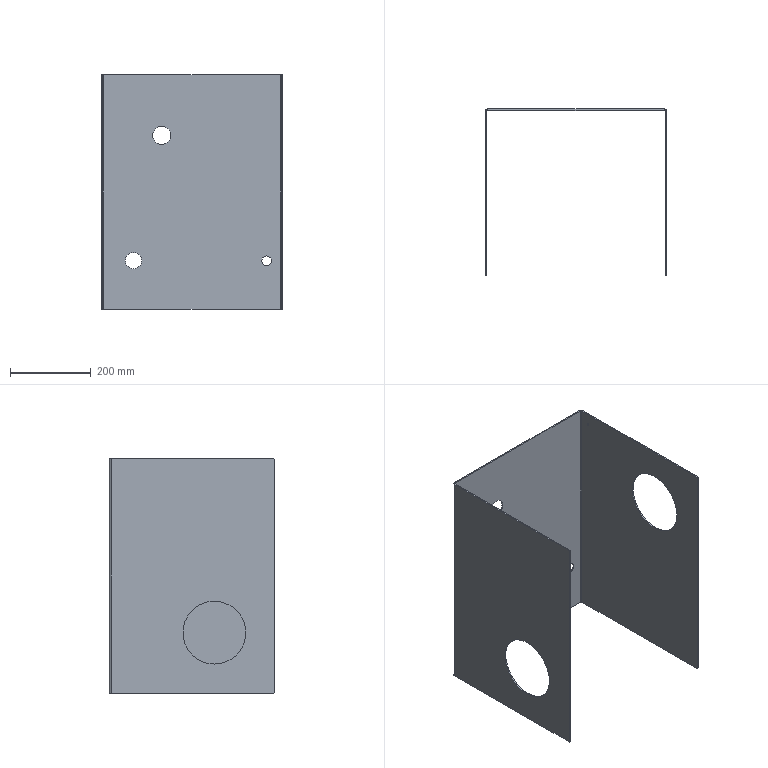Part | SolidWorks | features ICE 4, FlatPattern 1, SMBaseFlange 1, SheetMetal 1 | 1 solid | 38 faces | box 450 x 411 x 581 mm | volume 2075079 mm3 | cylinder 20 | plane 18 | commonest cylinder face diameters 6 x6 156 x4 5.2 x2 12 x2 24.2 x2 40.5 x2
STEP:
#1=CARTESIAN_POINT('',(3.,150.,72.));
#2=VERTEX_POINT('',#1);
#3=CARTESIAN_POINT('',(3.,150.,228.));
#4=VERTEX_POINT('',#3);
#5=CARTESIAN_POINT('',(3.,150.,150.));
#6=DIRECTION('',(-1.,0.,0.));
#7=DIRECTION('',(0.,0.,1.));
#8=AXIS2_PLACEMENT_3D('',#5,#6,#7);
#9=CIRCLE('',#8,78.);
#10=EDGE_CURVE('',#2,#4,#9,.T.);
#11=ORIENTED_EDGE('',*,*,#10,.F.);
#12=CARTESIAN_POINT('',(0.,150.,72.));
#13=VERTEX_POINT('',#12);
#14=CARTESIAN_POINT('',(10.,150.,72.));
#15=DIRECTION('',(-1.,0.,0.));
#16=VECTOR('',#15,1000.);
#17=LINE('',#14,#16);
#18=EDGE_CURVE('',#2,#13,#17,.T.);
#19=ORIENTED_EDGE('',*,*,#18,.T.);
#20=CARTESIAN_POINT('',(0.,150.,228.));
#21=VERTEX_POINT('',#20);
#22=CARTESIAN_POINT('',(0.,150.,150.));
#23=DIRECTION('',(-1.,0.,0.));
#24=DIRECTION('',(0.,0.,1.));
#25=AXIS2_PLACEMENT_3D('',#22,#23,#24);
#26=CIRCLE('',#25,78.);
#27=EDGE_CURVE('',#13,#21,#26,.T.);
#28=ORIENTED_EDGE('',*,*,#27,.T.);
#29=CARTESIAN_POINT('',(10.,150.,228.));
#30=DIRECTION('',(-1.,0.,0.));
#31=VECTOR('',#30,1000.);
#32=LINE('',#29,#31);
#33=EDGE_CURVE('',#4,#21,#32,.T.);
#34=ORIENTED_EDGE('',*,*,#33,.F.);
#35=EDGE_LOOP('',(#11,#19,#28,#34));
#36=FACE_OUTER_BOUND('',#35,.T.);
#37=CARTESIAN_POINT('',(10.,150.,150.));
#38=DIRECTION('',(-1.,0.,0.));
#39=DIRECTION('',(0.,0.,1.));
#40=AXIS2_PLACEMENT_3D('',#37,#38,#39);
#41=CYLINDRICAL_SURFACE('',#40,78.);
#42=ADVANCED_FACE('',(#36),#41,.F.);
#43=CARTESIAN_POINT('',(410.,408.,107.9));
#44=VERTEX_POINT('',#43);
#45=CARTESIAN_POINT('',(410.,408.,132.1));
#46=VERTEX_POINT('',#45);
#47=CARTESIAN_POINT('',(410.,408.,120.));
#48=DIRECTION('',(0.,1.,0.));
#49=DIRECTION('',(0.,0.,1.));
#50=AXIS2_PLACEMENT_3D('',#47,#48,#49);
#51=CIRCLE('',#50,12.1);
#52=EDGE_CURVE('',#44,#46,#51,.T.);
#53=ORIENTED_EDGE('',*,*,#52,.F.);
#54=CARTESIAN_POINT('',(410.,411.,107.9));
#55=VERTEX_POINT('',#54);
#56=CARTESIAN_POINT('',(410.,401.,107.9));
#57=DIRECTION('',(0.,1.,0.));
#58=VECTOR('',#57,1000.);
#59=LINE('',#56,#58);
#60=EDGE_CURVE('',#44,#55,#59,.T.);
#61=ORIENTED_EDGE('',*,*,#60,.T.);
#62=CARTESIAN_POINT('',(410.,411.,132.1));
#63=VERTEX_POINT('',#62);
#64=CARTESIAN_POINT('',(410.,411.,120.));
#65=DIRECTION('',(0.,1.,0.));
#66=DIRECTION('',(0.,0.,1.));
#67=AXIS2_PLACEMENT_3D('',#64,#65,#66);
#68=CIRCLE('',#67,12.1);
#69=EDGE_CURVE('',#55,#63,#68,.T.);
#70=ORIENTED_EDGE('',*,*,#69,.T.);
#71=CARTESIAN_POINT('',(410.,401.,132.1));
#72=DIRECTION('',(0.,1.,0.));
#73=VECTOR('',#72,1000.);
#74=LINE('',#71,#73);
#75=EDGE_CURVE('',#46,#63,#74,.T.);
#76=ORIENTED_EDGE('',*,*,#75,.F.);
#77=EDGE_LOOP('',(#53,#61,#70,#76));
#78=FACE_OUTER_BOUND('',#77,.T.);
#79=CARTESIAN_POINT('',(410.,401.,120.));
#80=DIRECTION('',(0.,1.,0.));
#81=DIRECTION('',(0.,0.,1.));
#82=AXIS2_PLACEMENT_3D('',#79,#80,#81);
#83=CYLINDRICAL_SURFACE('',#82,12.1);
#84=ADVANCED_FACE('',(#78),#83,.F.);
#85=CARTESIAN_POINT('',(80.,408.,99.75));
#86=VERTEX_POINT('',#85);
#87=CARTESIAN_POINT('',(80.,408.,140.25));
#88=VERTEX_POINT('',#87);
#89=CARTESIAN_POINT('',(80.,408.,120.));
#90=DIRECTION('',(0.,1.,0.));
#91=DIRECTION('',(0.,0.,1.));
#92=AXIS2_PLACEMENT_3D('',#89,#90,#91);
#93=CIRCLE('',#92,20.25);
#94=EDGE_CURVE('',#86,#88,#93,.T.);
#95=ORIENTED_EDGE('',*,*,#94,.F.);
#96=CARTESIAN_POINT('',(80.,411.,99.75));
#97=VERTEX_POINT('',#96);
#98=CARTESIAN_POINT('',(80.,401.,99.75));
#99=DIRECTION('',(0.,1.,0.));
#100=VECTOR('',#99,1000.);
#101=LINE('',#98,#100);
#102=EDGE_CURVE('',#86,#97,#101,.T.);
#103=ORIENTED_EDGE('',*,*,#102,.T.);
#104=CARTESIAN_POINT('',(80.,411.,140.25));
#105=VERTEX_POINT('',#104);
#106=CARTESIAN_POINT('',(80.,411.,120.));
#107=DIRECTION('',(0.,1.,0.));
#108=DIRECTION('',(0.,0.,1.));
#109=AXIS2_PLACEMENT_3D('',#106,#107,#108);
#110=CIRCLE('',#109,20.25);
#111=EDGE_CURVE('',#97,#105,#110,.T.);
#112=ORIENTED_EDGE('',*,*,#111,.T.);
#113=CARTESIAN_POINT('',(80.,401.,140.25));
#114=DIRECTION('',(0.,1.,0.));
#115=VECTOR('',#114,1000.);
#116=LINE('',#113,#115);
#117=EDGE_CURVE('',#88,#105,#116,.T.);
#118=ORIENTED_EDGE('',*,*,#117,.F.);
#119=EDGE_LOOP('',(#95,#103,#112,#118));
#120=FACE_OUTER_BOUND('',#119,.T.);
#121=CARTESIAN_POINT('',(80.,401.,120.));
#122=DIRECTION('',(0.,1.,0.));
#123=DIRECTION('',(0.,0.,1.));
#124=AXIS2_PLACEMENT_3D('',#121,#122,#123);
#125=CYLINDRICAL_SURFACE('',#124,20.25);
#126=ADVANCED_FACE('',(#120),#125,.F.);
#127=CARTESIAN_POINT('',(150.,408.,408.4));
#128=VERTEX_POINT('',#127);
#129=CARTESIAN_POINT('',(150.,408.,453.6));
#130=VERTEX_POINT('',#129);
#131=CARTESIAN_POINT('',(150.,408.,431.));
#132=DIRECTION('',(0.,1.,0.));
#133=DIRECTION('',(0.,0.,1.));
#134=AXIS2_PLACEMENT_3D('',#131,#132,#133);
#135=CIRCLE('',#134,22.6);
#136=EDGE_CURVE('',#128,#130,#135,.T.);
#137=ORIENTED_EDGE('',*,*,#136,.F.);
#138=CARTESIAN_POINT('',(150.,411.,408.4));
#139=VERTEX_POINT('',#138);
#140=CARTESIAN_POINT('',(150.,401.,408.4));
#141=DIRECTION('',(0.,1.,0.));
#142=VECTOR('',#141,1000.);
#143=LINE('',#140,#142);
#144=EDGE_CURVE('',#128,#139,#143,.T.);
#145=ORIENTED_EDGE('',*,*,#144,.T.);
#146=CARTESIAN_POINT('',(150.,411.,453.6));
#147=VERTEX_POINT('',#146);
#148=CARTESIAN_POINT('',(150.,411.,431.));
#149=DIRECTION('',(0.,1.,0.));
#150=DIRECTION('',(0.,0.,1.));
#151=AXIS2_PLACEMENT_3D('',#148,#149,#150);
#152=CIRCLE('',#151,22.6);
#153=EDGE_CURVE('',#139,#147,#152,.T.);
#154=ORIENTED_EDGE('',*,*,#153,.T.);
#155=CARTESIAN_POINT('',(150.,401.,453.6));
#156=DIRECTION('',(0.,1.,0.));
#157=VECTOR('',#156,1000.);
#158=LINE('',#155,#157);
#159=EDGE_CURVE('',#130,#147,#158,.T.);
#160=ORIENTED_EDGE('',*,*,#159,.F.);
#161=EDGE_LOOP('',(#137,#145,#154,#160));
#162=FACE_OUTER_BOUND('',#161,.T.);
#163=CARTESIAN_POINT('',(150.,401.,431.));
#164=DIRECTION('',(0.,1.,0.));
#165=DIRECTION('',(0.,0.,1.));
#166=AXIS2_PLACEMENT_3D('',#163,#164,#165);
#167=CYLINDRICAL_SURFACE('',#166,22.6);
#168=ADVANCED_FACE('',(#162),#167,.F.);
#169=CARTESIAN_POINT('',(447.,380.4,551.));
#170=VERTEX_POINT('',#169);
#171=CARTESIAN_POINT('',(447.,385.6,551.));
#172=VERTEX_POINT('',#171);
#173=CARTESIAN_POINT('',(447.,383.,551.));
#174=DIRECTION('',(1.,0.,0.));
#175=DIRECTION('',(0.,1.,0.));
#176=AXIS2_PLACEMENT_3D('',#173,#174,#175);
#177=CIRCLE('',#176,2.6);
#178=EDGE_CURVE('',#170,#172,#177,.T.);
#179=ORIENTED_EDGE('',*,*,#178,.F.);
#180=CARTESIAN_POINT('',(450.,380.4,551.));
#181=VERTEX_POINT('',#180);
#182=CARTESIAN_POINT('',(440.,380.4,551.));
#183=DIRECTION('',(1.,0.,0.));
#184=VECTOR('',#183,1000.);
#185=LINE('',#182,#184);
#186=EDGE_CURVE('',#170,#181,#185,.T.);
#187=ORIENTED_EDGE('',*,*,#186,.T.);
#188=CARTESIAN_POINT('',(450.,385.6,551.));
#189=VERTEX_POINT('',#188);
#190=CARTESIAN_POINT('',(450.,383.,551.));
#191=DIRECTION('',(1.,0.,0.));
#192=DIRECTION('',(0.,1.,0.));
#193=AXIS2_PLACEMENT_3D('',#190,#191,#192);
#194=CIRCLE('',#193,2.6);
#195=EDGE_CURVE('',#181,#189,#194,.T.);
#196=ORIENTED_EDGE('',*,*,#195,.T.);
#197=CARTESIAN_POINT('',(440.,385.6,551.));
#198=DIRECTION('',(1.,0.,0.));
#199=VECTOR('',#198,1000.);
#200=LINE('',#197,#199);
#201=EDGE_CURVE('',#172,#189,#200,.T.);
#202=ORIENTED_EDGE('',*,*,#201,.F.);
#203=EDGE_LOOP('',(#179,#187,#196,#202));
#204=FACE_OUTER_BOUND('',#203,.T.);
#205=CARTESIAN_POINT('',(440.,383.,551.));
#206=DIRECTION('',(1.,0.,0.));
#207=DIRECTION('',(0.,1.,0.));
#208=AXIS2_PLACEMENT_3D('',#205,#206,#207);
#209=CYLINDRICAL_SURFACE('',#208,2.6);
#210=ADVANCED_FACE('',(#204),#209,.F.);
#211=CARTESIAN_POINT('',(447.,72.,431.));
#212=VERTEX_POINT('',#211);
#213=CARTESIAN_POINT('',(447.,228.,431.));
#214=VERTEX_POINT('',#213);
#215=CARTESIAN_POINT('',(447.,150.,431.));
#216=DIRECTION('',(1.,0.,0.));
#217=DIRECTION('',(0.,1.,0.));
#218=AXIS2_PLACEMENT_3D('',#215,#216,#217);
#219=CIRCLE('',#218,78.);
#220=EDGE_CURVE('',#212,#214,#219,.T.);
#221=ORIENTED_EDGE('',*,*,#220,.F.);
#222=CARTESIAN_POINT('',(450.,72.,431.));
#223=VERTEX_POINT('',#222);
#224=CARTESIAN_POINT('',(440.,72.,431.));
#225=DIRECTION('',(1.,0.,0.));
#226=VECTOR('',#225,1000.);
#227=LINE('',#224,#226);
#228=EDGE_CURVE('',#212,#223,#227,.T.);
#229=ORIENTED_EDGE('',*,*,#228,.T.);
#230=CARTESIAN_POINT('',(450.,228.,431.));
#231=VERTEX_POINT('',#230);
#232=CARTESIAN_POINT('',(450.,150.,431.));
#233=DIRECTION('',(1.,0.,0.));
#234=DIRECTION('',(0.,1.,0.));
#235=AXIS2_PLACEMENT_3D('',#232,#233,#234);
#236=CIRCLE('',#235,78.);
#237=EDGE_CURVE('',#223,#231,#236,.T.);
#238=ORIENTED_EDGE('',*,*,#237,.T.);
#239=CARTESIAN_POINT('',(440.,228.,431.));
#240=DIRECTION('',(1.,0.,0.));
#241=VECTOR('',#240,1000.);
#242=LINE('',#239,#241);
#243=EDGE_CURVE('',#214,#231,#242,.T.);
#244=ORIENTED_EDGE('',*,*,#243,.F.);
#245=EDGE_LOOP('',(#221,#229,#238,#244));
#246=FACE_OUTER_BOUND('',#245,.T.);
#247=CARTESIAN_POINT('',(440.,150.,431.));
#248=DIRECTION('',(1.,0.,0.));
#249=DIRECTION('',(0.,1.,0.));
#250=AXIS2_PLACEMENT_3D('',#247,#248,#249);
#251=CYLINDRICAL_SURFACE('',#250,78.);
#252=ADVANCED_FACE('',(#246),#251,.F.);
#253=CARTESIAN_POINT('',(447.,383.,551.));
#254=DIRECTION('',(1.,0.,0.));
#255=DIRECTION('',(0.,1.,0.));
#256=AXIS2_PLACEMENT_3D('',#253,#254,#255);
#257=CIRCLE('',#256,2.6);
#258=EDGE_CURVE('',#172,#170,#257,.T.);
#259=ORIENTED_EDGE('',*,*,#258,.T.);
#260=ORIENTED_EDGE('',*,*,#178,.T.);
#261=EDGE_LOOP('',(#259,#260));
#262=FACE_BOUND('',#261,.T.);
#263=CARTESIAN_POINT('',(447.,150.,431.));
#264=DIRECTION('',(1.,0.,0.));
#265=DIRECTION('',(0.,1.,0.));
#266=AXIS2_PLACEMENT_3D('',#263,#264,#265);
#267=CIRCLE('',#266,78.);
#268=EDGE_CURVE('',#214,#212,#267,.T.);
#269=ORIENTED_EDGE('',*,*,#268,.T.);
#270=ORIENTED_EDGE('',*,*,#220,.T.);
#271=EDGE_LOOP('',(#269,#270));
#272=FACE_BOUND('',#271,.T.);
#273=CARTESIAN_POINT('',(447.,0.,578.));
#274=VERTEX_POINT('',#273);
#275=CARTESIAN_POINT('',(447.,3.,581.));
#276=VERTEX_POINT('',#275);
#277=CARTESIAN_POINT('',(447.,3.,578.));
#278=DIRECTION('',(-1.,0.,0.));
#279=DIRECTION('',(0.,1.,0.));
#280=AXIS2_PLACEMENT_3D('',#277,#278,#279);
#281=CIRCLE('',#280,3.);
#282=EDGE_CURVE('',#274,#276,#281,.T.);
#283=ORIENTED_EDGE('',*,*,#282,.T.);
#284=CARTESIAN_POINT('',(447.,405.,581.));
#285=VERTEX_POINT('',#284);
#286=CARTESIAN_POINT('',(447.,411.,581.));
#287=DIRECTION('',(0.,-1.,0.));
#288=VECTOR('',#287,1000.);
#289=LINE('',#286,#288);
#290=EDGE_CURVE('',#285,#276,#289,.T.);
#291=ORIENTED_EDGE('',*,*,#290,.F.);
#292=CARTESIAN_POINT('',(447.,405.,0.));
#293=VERTEX_POINT('',#292);
#294=CARTESIAN_POINT('',(447.,405.,581.));
#295=DIRECTION('',(0.,0.,-1.));
#296=VECTOR('',#295,1000.);
#297=LINE('',#294,#296);
#298=EDGE_CURVE('',#285,#293,#297,.T.);
#299=ORIENTED_EDGE('',*,*,#298,.T.);
#300=CARTESIAN_POINT('',(447.,3.,0.));
#301=VERTEX_POINT('',#300);
#302=CARTESIAN_POINT('',(447.,411.,0.));
#303=DIRECTION('',(0.,-1.,0.));
#304=VECTOR('',#303,1000.);
#305=LINE('',#302,#304);
#306=EDGE_CURVE('',#293,#301,#305,.T.);
#307=ORIENTED_EDGE('',*,*,#306,.T.);
#308=CARTESIAN_POINT('',(447.,0.,3.));
#309=VERTEX_POINT('',#308);
#310=CARTESIAN_POINT('',(447.,3.,3.));
#311=DIRECTION('',(-1.,0.,0.));
#312=DIRECTION('',(0.,1.,0.));
#313=AXIS2_PLACEMENT_3D('',#310,#311,#312);
#314=CIRCLE('',#313,3.);
#315=EDGE_CURVE('',#301,#309,#314,.T.);
#316=ORIENTED_EDGE('',*,*,#315,.T.);
#317=CARTESIAN_POINT('',(447.,0.,581.));
#318=DIRECTION('',(0.,0.,-1.));
#319=VECTOR('',#318,1000.);
#320=LINE('',#317,#319);
#321=EDGE_CURVE('',#274,#309,#320,.T.);
#322=ORIENTED_EDGE('',*,*,#321,.F.);
#323=EDGE_LOOP('',(#283,#291,#299,#307,#316,#322));
#324=FACE_OUTER_BOUND('',#323,.T.);
#325=CARTESIAN_POINT('',(447.,411.,581.));
#326=DIRECTION('',(1.,0.,0.));
#327=DIRECTION('',(0.,1.,0.));
#328=AXIS2_PLACEMENT_3D('',#325,#326,#327);
#329=PLANE('',#328);
#330=ADVANCED_FACE('',(#262,#272,#324),#329,.F.);
#331=CARTESIAN_POINT('',(450.,383.,551.));
#332=DIRECTION('',(1.,0.,0.));
#333=DIRECTION('',(0.,1.,0.));
#334=AXIS2_PLACEMENT_3D('',#331,#332,#333);
#335=CIRCLE('',#334,2.6);
#336=EDGE_CURVE('',#189,#181,#335,.T.);
#337=ORIENTED_EDGE('',*,*,#336,.F.);
#338=ORIENTED_EDGE('',*,*,#195,.F.);
#339=EDGE_LOOP('',(#337,#338));
#340=FACE_BOUND('',#339,.T.);
#341=CARTESIAN_POINT('',(450.,150.,431.));
#342=DIRECTION('',(1.,0.,0.));
#343=DIRECTION('',(0.,1.,0.));
#344=AXIS2_PLACEMENT_3D('',#341,#342,#343);
#345=CIRCLE('',#344,78.);
#346=EDGE_CURVE('',#231,#223,#345,.T.);
#347=ORIENTED_EDGE('',*,*,#346,.F.);
#348=ORIENTED_EDGE('',*,*,#237,.F.);
#349=EDGE_LOOP('',(#347,#348));
#350=FACE_BOUND('',#349,.T.);
#351=CARTESIAN_POINT('',(450.,405.,581.));
#352=VERTEX_POINT('',#351);
#353=CARTESIAN_POINT('',(450.,3.,581.));
#354=VERTEX_POINT('',#353);
#355=CARTESIAN_POINT('',(450.,411.,581.));
#356=DIRECTION('',(0.,-1.,0.));
#357=VECTOR('',#356,1000.);
#358=LINE('',#355,#357);
#359=EDGE_CURVE('',#352,#354,#358,.T.);
#360=ORIENTED_EDGE('',*,*,#359,.T.);
#361=CARTESIAN_POINT('',(450.,0.,578.));
#362=VERTEX_POINT('',#361);
#363=CARTESIAN_POINT('',(450.,3.,578.));
#364=DIRECTION('',(-1.,0.,0.));
#365=DIRECTION('',(0.,1.,0.));
#366=AXIS2_PLACEMENT_3D('',#363,#364,#365);
#367=CIRCLE('',#366,3.);
#368=EDGE_CURVE('',#362,#354,#367,.T.);
#369=ORIENTED_EDGE('',*,*,#368,.F.);
#370=CARTESIAN_POINT('',(450.,0.,3.));
#371=VERTEX_POINT('',#370);
#372=CARTESIAN_POINT('',(450.,0.,581.));
#373=DIRECTION('',(0.,0.,-1.));
#374=VECTOR('',#373,1000.);
#375=LINE('',#372,#374);
#376=EDGE_CURVE('',#362,#371,#375,.T.);
#377=ORIENTED_EDGE('',*,*,#376,.T.);
#378=CARTESIAN_POINT('',(450.,3.,0.));
#379=VERTEX_POINT('',#378);
#380=CARTESIAN_POINT('',(450.,3.,3.));
#381=DIRECTION('',(-1.,0.,0.));
#382=DIRECTION('',(0.,1.,0.));
#383=AXIS2_PLACEMENT_3D('',#380,#381,#382);
#384=CIRCLE('',#383,3.);
#385=EDGE_CURVE('',#379,#371,#384,.T.);
#386=ORIENTED_EDGE('',*,*,#385,.F.);
#387=CARTESIAN_POINT('',(450.,405.,0.));
#388=VERTEX_POINT('',#387);
#389=CARTESIAN_POINT('',(450.,411.,0.));
#390=DIRECTION('',(0.,-1.,0.));
#391=VECTOR('',#390,1000.);
#392=LINE('',#389,#391);
#393=EDGE_CURVE('',#388,#379,#392,.T.);
#394=ORIENTED_EDGE('',*,*,#393,.F.);
#395=CARTESIAN_POINT('',(450.,405.,581.));
#396=DIRECTION('',(0.,0.,-1.));
#397=VECTOR('',#396,1000.);
#398=LINE('',#395,#397);
#399=EDGE_CURVE('',#352,#388,#398,.T.);
#400=ORIENTED_EDGE('',*,*,#399,.F.);
#401=EDGE_LOOP('',(#360,#369,#377,#386,#394,#400));
#402=FACE_OUTER_BOUND('',#401,.T.);
#403=CARTESIAN_POINT('',(450.,411.,581.));
#404=DIRECTION('',(1.,0.,0.));
#405=DIRECTION('',(0.,1.,0.));
#406=AXIS2_PLACEMENT_3D('',#403,#404,#405);
#407=PLANE('',#406);
#408=ADVANCED_FACE('',(#340,#350,#402),#407,.T.);
#409=ORIENTED_EDGE('',*,*,#290,.T.);
#410=CARTESIAN_POINT('',(447.,3.,581.));
#411=DIRECTION('',(1.,0.,0.));
#412=VECTOR('',#411,1000.);
#413=LINE('',#410,#412);
#414=EDGE_CURVE('',#276,#354,#413,.T.);
#415=ORIENTED_EDGE('',*,*,#414,.T.);
#416=ORIENTED_EDGE('',*,*,#359,.F.);
#417=CARTESIAN_POINT('',(450.,405.,581.));
#418=DIRECTION('',(-1.,0.,0.));
#419=VECTOR('',#418,1000.);
#420=LINE('',#417,#419);
#421=EDGE_CURVE('',#352,#285,#420,.T.);
#422=ORIENTED_EDGE('',*,*,#421,.T.);
#423=EDGE_LOOP('',(#409,#415,#416,#422));
#424=FACE_OUTER_BOUND('',#423,.T.);
#425=CARTESIAN_POINT('',(444.,408.,581.));
#426=DIRECTION('',(0.,0.,1.));
#427=DIRECTION('',(1.,0.,0.));
#428=AXIS2_PLACEMENT_3D('',#425,#426,#427);
#429=PLANE('',#428);
#430=ADVANCED_FACE('',(#424),#429,.T.);
#431=CARTESIAN_POINT('',(447.,0.,578.));
#432=DIRECTION('',(1.,0.,0.));
#433=VECTOR('',#432,1000.);
#434=LINE('',#431,#433);
#435=EDGE_CURVE('',#274,#362,#434,.T.);
#436=ORIENTED_EDGE('',*,*,#435,.F.);
#437=ORIENTED_EDGE('',*,*,#321,.T.);
#438=CARTESIAN_POINT('',(447.,0.,3.));
#439=DIRECTION('',(1.,0.,0.));
#440=VECTOR('',#439,1000.);
#441=LINE('',#438,#440);
#442=EDGE_CURVE('',#309,#371,#441,.T.);
#443=ORIENTED_EDGE('',*,*,#442,.T.);
#444=ORIENTED_EDGE('',*,*,#376,.F.);
#445=EDGE_LOOP('',(#436,#437,#443,#444));
#446=FACE_OUTER_BOUND('',#445,.T.);
#447=CARTESIAN_POINT('',(450.,0.,581.));
#448=DIRECTION('',(0.,-1.,0.));
#449=DIRECTION('',(1.,0.,0.));
#450=AXIS2_PLACEMENT_3D('',#447,#448,#449);
#451=PLANE('',#450);
#452=ADVANCED_FACE('',(#446),#451,.T.);
#453=CARTESIAN_POINT('',(447.,3.,0.));
#454=DIRECTION('',(1.,0.,0.));
#455=VECTOR('',#454,1000.);
#456=LINE('',#453,#455);
#457=EDGE_CURVE('',#301,#379,#456,.T.);
#458=ORIENTED_EDGE('',*,*,#457,.F.);
#459=ORIENTED_EDGE('',*,*,#306,.F.);
#460=CARTESIAN_POINT('',(447.,405.,0.));
#461=DIRECTION('',(1.,0.,0.));
#462=VECTOR('',#461,1000.);
#463=LINE('',#460,#462);
#464=EDGE_CURVE('',#293,#388,#463,.T.);
#465=ORIENTED_EDGE('',*,*,#464,.T.);
#466=ORIENTED_EDGE('',*,*,#393,.T.);
#467=EDGE_LOOP('',(#458,#459,#465,#466));
#468=FACE_OUTER_BOUND('',#467,.T.);
#469=CARTESIAN_POINT('',(444.,405.,0.));
#470=DIRECTION('',(0.,0.,1.));
#471=DIRECTION('',(1.,0.,0.));
#472=AXIS2_PLACEMENT_3D('',#469,#470,#471);
#473=PLANE('',#472);
#474=ADVANCED_FACE('',(#468),#473,.F.);
#475=CARTESIAN_POINT('',(0.,150.,150.));
#476=DIRECTION('',(-1.,0.,0.));
#477=DIRECTION('',(0.,0.,1.));
#478=AXIS2_PLACEMENT_3D('',#475,#476,#477);
#479=CIRCLE('',#478,78.);
#480=EDGE_CURVE('',#21,#13,#479,.T.);
#481=ORIENTED_EDGE('',*,*,#480,.F.);
#482=ORIENTED_EDGE('',*,*,#27,.F.);
#483=EDGE_LOOP('',(#481,#482));
#484=FACE_BOUND('',#483,.T.);
#485=CARTESIAN_POINT('',(0.,0.,578.));
#486=VERTEX_POINT('',#485);
#487=CARTESIAN_POINT('',(0.,0.,3.));
#488=VERTEX_POINT('',#487);
#489=CARTESIAN_POINT('',(0.,0.,581.));
#490=DIRECTION('',(0.,0.,-1.));
#491=VECTOR('',#490,1000.);
#492=LINE('',#489,#491);
#493=EDGE_CURVE('',#486,#488,#492,.T.);
#494=ORIENTED_EDGE('',*,*,#493,.F.);
#495=CARTESIAN_POINT('',(0.,3.,581.));
#496=VERTEX_POINT('',#495);
#497=CARTESIAN_POINT('',(0.,3.,578.));
#498=DIRECTION('',(1.,0.,0.));
#499=DIRECTION('',(0.,0.,1.));
#500=AXIS2_PLACEMENT_3D('',#497,#498,#499);
#501=CIRCLE('',#500,3.);
#502=EDGE_CURVE('',#496,#486,#501,.T.);
#503=ORIENTED_EDGE('',*,*,#502,.F.);
#504=CARTESIAN_POINT('',(0.,405.,581.));
#505=VERTEX_POINT('',#504);
#506=CARTESIAN_POINT('',(0.,0.,581.));
#507=DIRECTION('',(0.,1.,0.));
#508=VECTOR('',#507,1000.);
#509=LINE('',#506,#508);
#510=EDGE_CURVE('',#496,#505,#509,.T.);
#511=ORIENTED_EDGE('',*,*,#510,.T.);
#512=CARTESIAN_POINT('',(0.,405.,0.));
#513=VERTEX_POINT('',#512);
#514=CARTESIAN_POINT('',(0.,405.,581.));
#515=DIRECTION('',(0.,0.,-1.));
#516=VECTOR('',#515,1000.);
#517=LINE('',#514,#516);
#518=EDGE_CURVE('',#505,#513,#517,.T.);
#519=ORIENTED_EDGE('',*,*,#518,.T.);
#520=CARTESIAN_POINT('',(0.,3.,0.));
#521=VERTEX_POINT('',#520);
#522=CARTESIAN_POINT('',(0.,0.,0.));
#523=DIRECTION('',(0.,1.,0.));
#524=VECTOR('',#523,1000.);
#525=LINE('',#522,#524);
#526=EDGE_CURVE('',#521,#513,#525,.T.);
#527=ORIENTED_EDGE('',*,*,#526,.F.);
#528=CARTESIAN_POINT('',(0.,3.,3.));
#529=DIRECTION('',(1.,0.,0.));
#530=DIRECTION('',(0.,0.,1.));
#531=AXIS2_PLACEMENT_3D('',#528,#529,#530);
#532=CIRCLE('',#531,3.);
#533=EDGE_CURVE('',#488,#521,#532,.T.);
#534=ORIENTED_EDGE('',*,*,#533,.F.);
#535=EDGE_LOOP('',(#494,#503,#511,#519,#527,#534));
#536=FACE_OUTER_BOUND('',#535,.T.);
#537=CARTESIAN_POINT('',(0.,0.,581.));
#538=DIRECTION('',(-1.,0.,0.));
#539=DIRECTION('',(0.,0.,1.));
#540=AXIS2_PLACEMENT_3D('',#537,#538,#539);
#541=PLANE('',#540);
#542=ADVANCED_FACE('',(#484,#536),#541,.T.);
#543=CARTESIAN_POINT('',(3.,150.,150.));
#544=DIRECTION('',(-1.,0.,0.));
#545=DIRECTION('',(0.,0.,1.));
#546=AXIS2_PLACEMENT_3D('',#543,#544,#545);
#547=CIRCLE('',#546,78.);
#548=EDGE_CURVE('',#4,#2,#547,.T.);
#549=ORIENTED_EDGE('',*,*,#548,.T.);
#550=ORIENTED_EDGE('',*,*,#10,.T.);
#551=EDGE_LOOP('',(#549,#550));
#552=FACE_BOUND('',#551,.T.);
#553=CARTESIAN_POINT('',(3.,3.,581.));
#554=VERTEX_POINT('',#553);
#555=CARTESIAN_POINT('',(3.,0.,578.));
#556=VERTEX_POINT('',#555);
#557=CARTESIAN_POINT('',(3.,3.,578.));
#558=DIRECTION('',(1.,0.,0.));
#559=DIRECTION('',(0.,0.,1.));
#560=AXIS2_PLACEMENT_3D('',#557,#558,#559);
#561=CIRCLE('',#560,3.);
#562=EDGE_CURVE('',#554,#556,#561,.T.);
#563=ORIENTED_EDGE('',*,*,#562,.T.);
#564=CARTESIAN_POINT('',(3.,0.,3.));
#565=VERTEX_POINT('',#564);
#566=CARTESIAN_POINT('',(3.,0.,581.));
#567=DIRECTION('',(0.,0.,-1.));
#568=VECTOR('',#567,1000.);
#569=LINE('',#566,#568);
#570=EDGE_CURVE('',#556,#565,#569,.T.);
#571=ORIENTED_EDGE('',*,*,#570,.T.);
#572=CARTESIAN_POINT('',(3.,3.,0.));
#573=VERTEX_POINT('',#572);
#574=CARTESIAN_POINT('',(3.,3.,3.));
#575=DIRECTION('',(1.,0.,0.));
#576=DIRECTION('',(0.,0.,1.));
#577=AXIS2_PLACEMENT_3D('',#574,#575,#576);
#578=CIRCLE('',#577,3.);
#579=EDGE_CURVE('',#565,#573,#578,.T.);
#580=ORIENTED_EDGE('',*,*,#579,.T.);
#581=CARTESIAN_POINT('',(3.,405.,0.));
#582=VERTEX_POINT('',#581);
#583=CARTESIAN_POINT('',(3.,0.,0.));
#584=DIRECTION('',(0.,1.,0.));
#585=VECTOR('',#584,1000.);
#586=LINE('',#583,#585);
#587=EDGE_CURVE('',#573,#582,#586,.T.);
#588=ORIENTED_EDGE('',*,*,#587,.T.);
#589=CARTESIAN_POINT('',(3.,405.,581.));
#590=VERTEX_POINT('',#589);
#591=CARTESIAN_POINT('',(3.,405.,581.));
#592=DIRECTION('',(0.,0.,-1.));
#593=VECTOR('',#592,1000.);
#594=LINE('',#591,#593);
#595=EDGE_CURVE('',#590,#582,#594,.T.);
#596=ORIENTED_EDGE('',*,*,#595,.F.);
#597=CARTESIAN_POINT('',(3.,0.,581.));
#598=DIRECTION('',(0.,1.,0.));
#599=VECTOR('',#598,1000.);
#600=LINE('',#597,#599);
#601=EDGE_CURVE('',#554,#590,#600,.T.);
#602=ORIENTED_EDGE('',*,*,#601,.F.);
#603=EDGE_LOOP('',(#563,#571,#580,#588,#596,#602));
#604=FACE_OUTER_BOUND('',#603,.T.);
#605=CARTESIAN_POINT('',(3.,0.,581.));
#606=DIRECTION('',(-1.,0.,0.));
#607=DIRECTION('',(0.,0.,1.));
#608=AXIS2_PLACEMENT_3D('',#605,#606,#607);
#609=PLANE('',#608);
#610=ADVANCED_FACE('',(#552,#604),#609,.F.);
#611=ORIENTED_EDGE('',*,*,#570,.F.);
#612=CARTESIAN_POINT('',(3.,0.,578.));
#613=DIRECTION('',(-1.,0.,0.));
#614=VECTOR('',#613,1000.);
#615=LINE('',#612,#614);
#616=EDGE_CURVE('',#556,#486,#615,.T.);
#617=ORIENTED_EDGE('',*,*,#616,.T.);
#618=ORIENTED_EDGE('',*,*,#493,.T.);
#619=CARTESIAN_POINT('',(3.,0.,3.));
#620=DIRECTION('',(-1.,0.,0.));
#621=VECTOR('',#620,1000.);
#622=LINE('',#619,#621);
#623=EDGE_CURVE('',#565,#488,#622,.T.);
#624=ORIENTED_EDGE('',*,*,#623,.F.);
#625=EDGE_LOOP('',(#611,#617,#618,#624));
#626=FACE_OUTER_BOUND('',#625,.T.);
#627=CARTESIAN_POINT('',(3.,0.,581.));
#628=DIRECTION('',(0.,-1.,0.));
#629=DIRECTION('',(0.,0.,-1.));
#630=AXIS2_PLACEMENT_3D('',#627,#628,#629);
#631=PLANE('',#630);
#632=ADVANCED_FACE('',(#626),#631,.T.);
#633=ORIENTED_EDGE('',*,*,#587,.F.);
#634=CARTESIAN_POINT('',(3.,3.,0.));
#635=DIRECTION('',(-1.,0.,0.));
#636=VECTOR('',#635,1000.);
#637=LINE('',#634,#636);
#638=EDGE_CURVE('',#573,#521,#637,.T.);
#639=ORIENTED_EDGE('',*,*,#638,.T.);
#640=ORIENTED_EDGE('',*,*,#526,.T.);
#641=CARTESIAN_POINT('',(0.,405.,0.));
#642=DIRECTION('',(1.,0.,0.));
#643=VECTOR('',#642,1000.);
#644=LINE('',#641,#643);
#645=EDGE_CURVE('',#513,#582,#644,.T.);
#646=ORIENTED_EDGE('',*,*,#645,.T.);
#647=EDGE_LOOP('',(#633,#639,#640,#646));
#648=FACE_OUTER_BOUND('',#647,.T.);
#649=CARTESIAN_POINT('',(6.,408.,0.));
#650=DIRECTION('',(0.,0.,-1.));
#651=DIRECTION('',(-1.,0.,0.));
#652=AXIS2_PLACEMENT_3D('',#649,#650,#651);
#653=PLANE('',#652);
#654=ADVANCED_FACE('',(#648),#653,.T.);
#655=CARTESIAN_POINT('',(6.,411.,581.));
#656=VERTEX_POINT('',#655);
#657=CARTESIAN_POINT('',(6.,408.,581.));
#658=VERTEX_POINT('',#657);
#659=CARTESIAN_POINT('',(6.,411.,581.));
#660=DIRECTION('',(0.,-1.,0.));
#661=VECTOR('',#660,1000.);
#662=LINE('',#659,#661);
#663=EDGE_CURVE('',#656,#658,#662,.T.);
#664=ORIENTED_EDGE('',*,*,#663,.F.);
#665=CARTESIAN_POINT('',(6.,405.,581.));
#666=DIRECTION('',(0.,0.,-1.));
#667=DIRECTION('',(1.,0.,0.));
#668=AXIS2_PLACEMENT_3D('',#665,#666,#667);
#669=CIRCLE('',#668,6.);
#670=EDGE_CURVE('',#505,#656,#669,.T.);
#671=ORIENTED_EDGE('',*,*,#670,.F.);
#672=CARTESIAN_POINT('',(3.,405.,581.));
#673=DIRECTION('',(-1.,0.,0.));
#674=VECTOR('',#673,1000.);
#675=LINE('',#672,#674);
#676=EDGE_CURVE('',#590,#505,#675,.T.);
#677=ORIENTED_EDGE('',*,*,#676,.F.);
#678=CARTESIAN_POINT('',(6.,405.,581.));
#679=DIRECTION('',(0.,0.,-1.));
#680=DIRECTION('',(1.,0.,0.));
#681=AXIS2_PLACEMENT_3D('',#678,#679,#680);
#682=CIRCLE('',#681,3.);
#683=EDGE_CURVE('',#590,#658,#682,.T.);
#684=ORIENTED_EDGE('',*,*,#683,.T.);
#685=EDGE_LOOP('',(#664,#671,#677,#684));
#686=FACE_OUTER_BOUND('',#685,.T.);
#687=CARTESIAN_POINT('',(6.,411.,581.));
#688=DIRECTION('',(0.,0.,1.));
#689=DIRECTION('',(1.,0.,0.));
#690=AXIS2_PLACEMENT_3D('',#687,#688,#689);
#691=PLANE('',#690);
#692=ADVANCED_FACE('',(#686),#691,.T.);
#693=CARTESIAN_POINT('',(444.,411.,581.));
#694=VERTEX_POINT('',#693);
#695=CARTESIAN_POINT('',(0.,411.,581.));
#696=DIRECTION('',(1.,0.,0.));
#697=VECTOR('',#696,1000.);
#698=LINE('',#695,#697);
#699=EDGE_CURVE('',#656,#694,#698,.T.);
#700=ORIENTED_EDGE('',*,*,#699,.F.);
#701=ORIENTED_EDGE('',*,*,#663,.T.);
#702=CARTESIAN_POINT('',(444.,408.,581.));
#703=VERTEX_POINT('',#702);
#704=CARTESIAN_POINT('',(0.,408.,581.));
#705=DIRECTION('',(1.,0.,0.));
#706=VECTOR('',#705,1000.);
#707=LINE('',#704,#706);
#708=EDGE_CURVE('',#658,#703,#707,.T.);
#709=ORIENTED_EDGE('',*,*,#708,.T.);
#710=CARTESIAN_POINT('',(444.,408.,581.));
#711=DIRECTION('',(0.,1.,0.));
#712=VECTOR('',#711,1000.);
#713=LINE('',#710,#712);
#714=EDGE_CURVE('',#703,#694,#713,.T.);
#715=ORIENTED_EDGE('',*,*,#714,.T.);
#716=EDGE_LOOP('',(#700,#701,#709,#715));
#717=FACE_OUTER_BOUND('',#716,.T.);
#718=CARTESIAN_POINT('',(3.,405.,581.));
#719=DIRECTION('',(0.,0.,1.));
#720=DIRECTION('',(1.,0.,0.));
#721=AXIS2_PLACEMENT_3D('',#718,#719,#720);
#722=PLANE('',#721);
#723=ADVANCED_FACE('',(#717),#722,.T.);
#724=ORIENTED_EDGE('',*,*,#645,.F.);
#725=CARTESIAN_POINT('',(6.,411.,0.));
#726=VERTEX_POINT('',#725);
#727=CARTESIAN_POINT('',(6.,405.,0.));
#728=DIRECTION('',(0.,0.,-1.));
#729=DIRECTION('',(1.,0.,0.));
#730=AXIS2_PLACEMENT_3D('',#727,#728,#729);
#731=CIRCLE('',#730,6.);
#732=EDGE_CURVE('',#513,#726,#731,.T.);
#733=ORIENTED_EDGE('',*,*,#732,.T.);
#734=CARTESIAN_POINT('',(6.,408.,0.));
#735=VERTEX_POINT('',#734);
#736=CARTESIAN_POINT('',(6.,408.,0.));
#737=DIRECTION('',(0.,1.,0.));
#738=VECTOR('',#737,1000.);
#739=LINE('',#736,#738);
#740=EDGE_CURVE('',#735,#726,#739,.T.);
#741=ORIENTED_EDGE('',*,*,#740,.F.);
#742=CARTESIAN_POINT('',(6.,405.,0.));
#743=DIRECTION('',(0.,0.,-1.));
#744=DIRECTION('',(1.,0.,0.));
#745=AXIS2_PLACEMENT_3D('',#742,#743,#744);
#746=CIRCLE('',#745,3.);
#747=EDGE_CURVE('',#582,#735,#746,.T.);
#748=ORIENTED_EDGE('',*,*,#747,.F.);
#749=EDGE_LOOP('',(#724,#733,#741,#748));
#750=FACE_OUTER_BOUND('',#749,.T.);
#751=CARTESIAN_POINT('',(0.,405.,0.));
#752=DIRECTION('',(0.,0.,-1.));
#753=DIRECTION('',(-1.,0.,0.));
#754=AXIS2_PLACEMENT_3D('',#751,#752,#753);
#755=PLANE('',#754);
#756=ADVANCED_FACE('',(#750),#755,.T.);
#757=ORIENTED_EDGE('',*,*,#421,.F.);
#758=CARTESIAN_POINT('',(444.,405.,581.));
#759=DIRECTION('',(0.,0.,-1.));
#760=DIRECTION('',(1.,0.,0.));
#761=AXIS2_PLACEMENT_3D('',#758,#759,#760);
#762=CIRCLE('',#761,6.);
#763=EDGE_CURVE('',#694,#352,#762,.T.);
#764=ORIENTED_EDGE('',*,*,#763,.F.);
#765=ORIENTED_EDGE('',*,*,#714,.F.);
#766=CARTESIAN_POINT('',(444.,405.,581.));
#767=DIRECTION('',(0.,0.,-1.));
#768=DIRECTION('',(1.,0.,0.));
#769=AXIS2_PLACEMENT_3D('',#766,#767,#768);
#770=CIRCLE('',#769,3.);
#771=EDGE_CURVE('',#703,#285,#770,.T.);
#772=ORIENTED_EDGE('',*,*,#771,.T.);
#773=EDGE_LOOP('',(#757,#764,#765,#772));
#774=FACE_OUTER_BOUND('',#773,.T.);
#775=CARTESIAN_POINT('',(450.,405.,581.));
#776=DIRECTION('',(0.,0.,1.));
#777=DIRECTION('',(1.,0.,0.));
#778=AXIS2_PLACEMENT_3D('',#775,#776,#777);
#779=PLANE('',#778);
#780=ADVANCED_FACE('',(#774),#779,.T.);
#781=CARTESIAN_POINT('',(444.,411.,0.));
#782=VERTEX_POINT('',#781);
#783=CARTESIAN_POINT('',(444.,408.,0.));
#784=VERTEX_POINT('',#783);
#785=CARTESIAN_POINT('',(444.,411.,0.));
#786=DIRECTION('',(0.,-1.,0.));
#787=VECTOR('',#786,1000.);
#788=LINE('',#785,#787);
#789=EDGE_CURVE('',#782,#784,#788,.T.);
#790=ORIENTED_EDGE('',*,*,#789,.F.);
#791=CARTESIAN_POINT('',(444.,405.,0.));
#792=DIRECTION('',(0.,0.,-1.));
#793=DIRECTION('',(1.,0.,0.));
#794=AXIS2_PLACEMENT_3D('',#791,#792,#793);
#795=CIRCLE('',#794,6.);
#796=EDGE_CURVE('',#782,#388,#795,.T.);
#797=ORIENTED_EDGE('',*,*,#796,.T.);
#798=ORIENTED_EDGE('',*,*,#464,.F.);
#799=CARTESIAN_POINT('',(444.,405.,0.));
#800=DIRECTION('',(0.,0.,-1.));
#801=DIRECTION('',(1.,0.,0.));
#802=AXIS2_PLACEMENT_3D('',#799,#800,#801);
#803=CIRCLE('',#802,3.);
#804=EDGE_CURVE('',#784,#293,#803,.T.);
#805=ORIENTED_EDGE('',*,*,#804,.F.);
#806=EDGE_LOOP('',(#790,#797,#798,#805));
#807=FACE_OUTER_BOUND('',#806,.T.);
#808=CARTESIAN_POINT('',(444.,411.,0.));
#809=DIRECTION('',(0.,0.,-1.));
#810=DIRECTION('',(-1.,0.,0.));
#811=AXIS2_PLACEMENT_3D('',#808,#809,#810);
#812=PLANE('',#811);
#813=ADVANCED_FACE('',(#807),#812,.T.);
#814=CARTESIAN_POINT('',(0.,411.,0.));
#815=DIRECTION('',(1.,0.,0.));
#816=VECTOR('',#815,1000.);
#817=LINE('',#814,#816);
#818=EDGE_CURVE('',#726,#782,#817,.T.);
#819=ORIENTED_EDGE('',*,*,#818,.T.);
#820=ORIENTED_EDGE('',*,*,#789,.T.);
#821=CARTESIAN_POINT('',(0.,408.,0.));
#822=DIRECTION('',(1.,0.,0.));
#823=VECTOR('',#822,1000.);
#824=LINE('',#821,#823);
#825=EDGE_CURVE('',#735,#784,#824,.T.);
#826=ORIENTED_EDGE('',*,*,#825,.F.);
#827=ORIENTED_EDGE('',*,*,#740,.T.);
#828=EDGE_LOOP('',(#819,#820,#826,#827));
#829=FACE_OUTER_BOUND('',#828,.T.);
#830=CARTESIAN_POINT('',(447.,405.,0.));
#831=DIRECTION('',(0.,0.,-1.));
#832=DIRECTION('',(-1.,0.,0.));
#833=AXIS2_PLACEMENT_3D('',#830,#831,#832);
#834=PLANE('',#833);
#835=ADVANCED_FACE('',(#829),#834,.T.);
#836=ORIENTED_EDGE('',*,*,#796,.F.);
#837=CARTESIAN_POINT('',(444.,411.,581.));
#838=DIRECTION('',(0.,0.,-1.));
#839=VECTOR('',#838,1000.);
#840=LINE('',#837,#839);
#841=EDGE_CURVE('',#694,#782,#840,.T.);
#842=ORIENTED_EDGE('',*,*,#841,.F.);
#843=ORIENTED_EDGE('',*,*,#763,.T.);
#844=ORIENTED_EDGE('',*,*,#399,.T.);
#845=EDGE_LOOP('',(#836,#842,#843,#844));
#846=FACE_OUTER_BOUND('',#845,.T.);
#847=CARTESIAN_POINT('',(444.,405.,581.));
#848=DIRECTION('',(0.,0.,-1.));
#849=DIRECTION('',(-1.,0.,0.));
#850=AXIS2_PLACEMENT_3D('',#847,#848,#849);
#851=CYLINDRICAL_SURFACE('',#850,6.);
#852=ADVANCED_FACE('',(#846),#851,.T.);
#853=CARTESIAN_POINT('',(410.,411.,120.));
#854=DIRECTION('',(0.,1.,0.));
#855=DIRECTION('',(0.,0.,1.));
#856=AXIS2_PLACEMENT_3D('',#853,#854,#855);
#857=CIRCLE('',#856,12.1);
#858=EDGE_CURVE('',#63,#55,#857,.T.);
#859=ORIENTED_EDGE('',*,*,#858,.F.);
#860=ORIENTED_EDGE('',*,*,#69,.F.);
#861=EDGE_LOOP('',(#859,#860));
#862=FACE_BOUND('',#861,.T.);
#863=CARTESIAN_POINT('',(80.,411.,120.));
#864=DIRECTION('',(0.,1.,0.));
#865=DIRECTION('',(0.,0.,1.));
#866=AXIS2_PLACEMENT_3D('',#863,#864,#865);
#867=CIRCLE('',#866,20.25);
#868=EDGE_CURVE('',#105,#97,#867,.T.);
#869=ORIENTED_EDGE('',*,*,#868,.F.);
#870=ORIENTED_EDGE('',*,*,#111,.F.);
#871=EDGE_LOOP('',(#869,#870));
#872=FACE_BOUND('',#871,.T.);
#873=CARTESIAN_POINT('',(150.,411.,431.));
#874=DIRECTION('',(0.,1.,0.));
#875=DIRECTION('',(0.,0.,1.));
#876=AXIS2_PLACEMENT_3D('',#873,#874,#875);
#877=CIRCLE('',#876,22.6);
#878=EDGE_CURVE('',#147,#139,#877,.T.);
#879=ORIENTED_EDGE('',*,*,#878,.F.);
#880=ORIENTED_EDGE('',*,*,#153,.F.);
#881=EDGE_LOOP('',(#879,#880));
#882=FACE_BOUND('',#881,.T.);
#883=ORIENTED_EDGE('',*,*,#818,.F.);
#884=CARTESIAN_POINT('',(6.,411.,581.));
#885=DIRECTION('',(0.,0.,-1.));
#886=VECTOR('',#885,1000.);
#887=LINE('',#884,#886);
#888=EDGE_CURVE('',#656,#726,#887,.T.);
#889=ORIENTED_EDGE('',*,*,#888,.F.);
#890=ORIENTED_EDGE('',*,*,#699,.T.);
#891=ORIENTED_EDGE('',*,*,#841,.T.);
#892=EDGE_LOOP('',(#883,#889,#890,#891));
#893=FACE_OUTER_BOUND('',#892,.T.);
#894=CARTESIAN_POINT('',(0.,411.,581.));
#895=DIRECTION('',(0.,1.,0.));
#896=DIRECTION('',(0.,0.,1.));
#897=AXIS2_PLACEMENT_3D('',#894,#895,#896);
#898=PLANE('',#897);
#899=ADVANCED_FACE('',(#862,#872,#882,#893),#898,.T.);
#900=ORIENTED_EDGE('',*,*,#732,.F.);
#901=ORIENTED_EDGE('',*,*,#518,.F.);
#902=ORIENTED_EDGE('',*,*,#670,.T.);
#903=ORIENTED_EDGE('',*,*,#888,.T.);
#904=EDGE_LOOP('',(#900,#901,#902,#903));
#905=FACE_OUTER_BOUND('',#904,.T.);
#906=CARTESIAN_POINT('',(6.,405.,581.));
#907=DIRECTION('',(0.,0.,-1.));
#908=DIRECTION('',(-1.,0.,0.));
#909=AXIS2_PLACEMENT_3D('',#906,#907,#908);
#910=CYLINDRICAL_SURFACE('',#909,6.);
#911=ADVANCED_FACE('',(#905),#910,.T.);
#912=ORIENTED_EDGE('',*,*,#747,.T.);
#913=CARTESIAN_POINT('',(6.,408.,581.));
#914=DIRECTION('',(0.,0.,-1.));
#915=VECTOR('',#914,1000.);
#916=LINE('',#913,#915);
#917=EDGE_CURVE('',#658,#735,#916,.T.);
#918=ORIENTED_EDGE('',*,*,#917,.F.);
#919=ORIENTED_EDGE('',*,*,#683,.F.);
#920=ORIENTED_EDGE('',*,*,#595,.T.);
#921=EDGE_LOOP('',(#912,#918,#919,#920));
#922=FACE_OUTER_BOUND('',#921,.T.);
#923=CARTESIAN_POINT('',(6.,405.,581.));
#924=DIRECTION('',(0.,0.,-1.));
#925=DIRECTION('',(-1.,0.,0.));
#926=AXIS2_PLACEMENT_3D('',#923,#924,#925);
#927=CYLINDRICAL_SURFACE('',#926,3.);
#928=ADVANCED_FACE('',(#922),#927,.F.);
#929=CARTESIAN_POINT('',(410.,408.,120.));
#930=DIRECTION('',(0.,1.,0.));
#931=DIRECTION('',(0.,0.,1.));
#932=AXIS2_PLACEMENT_3D('',#929,#930,#931);
#933=CIRCLE('',#932,12.1);
#934=EDGE_CURVE('',#46,#44,#933,.T.);
#935=ORIENTED_EDGE('',*,*,#934,.T.);
#936=ORIENTED_EDGE('',*,*,#52,.T.);
#937=EDGE_LOOP('',(#935,#936));
#938=FACE_BOUND('',#937,.T.);
#939=CARTESIAN_POINT('',(80.,408.,120.));
#940=DIRECTION('',(0.,1.,0.));
#941=DIRECTION('',(0.,0.,1.));
#942=AXIS2_PLACEMENT_3D('',#939,#940,#941);
#943=CIRCLE('',#942,20.25);
#944=EDGE_CURVE('',#88,#86,#943,.T.);
#945=ORIENTED_EDGE('',*,*,#944,.T.);
#946=ORIENTED_EDGE('',*,*,#94,.T.);
#947=EDGE_LOOP('',(#945,#946));
#948=FACE_BOUND('',#947,.T.);
#949=CARTESIAN_POINT('',(150.,408.,431.));
#950=DIRECTION('',(0.,1.,0.));
#951=DIRECTION('',(0.,0.,1.));
#952=AXIS2_PLACEMENT_3D('',#949,#950,#951);
#953=CIRCLE('',#952,22.6);
#954=EDGE_CURVE('',#130,#128,#953,.T.);
#955=ORIENTED_EDGE('',*,*,#954,.T.);
#956=ORIENTED_EDGE('',*,*,#136,.T.);
#957=EDGE_LOOP('',(#955,#956));
#958=FACE_BOUND('',#957,.T.);
#959=ORIENTED_EDGE('',*,*,#825,.T.);
#960=CARTESIAN_POINT('',(444.,408.,581.));
#961=DIRECTION('',(0.,0.,-1.));
#962=VECTOR('',#961,1000.);
#963=LINE('',#960,#962);
#964=EDGE_CURVE('',#703,#784,#963,.T.);
#965=ORIENTED_EDGE('',*,*,#964,.F.);
#966=ORIENTED_EDGE('',*,*,#708,.F.);
#967=ORIENTED_EDGE('',*,*,#917,.T.);
#968=EDGE_LOOP('',(#959,#965,#966,#967));
#969=FACE_OUTER_BOUND('',#968,.T.);
#970=CARTESIAN_POINT('',(0.,408.,581.));
#971=DIRECTION('',(0.,1.,0.));
#972=DIRECTION('',(0.,0.,1.));
#973=AXIS2_PLACEMENT_3D('',#970,#971,#972);
#974=PLANE('',#973);
#975=ADVANCED_FACE('',(#938,#948,#958,#969),#974,.F.);
#976=ORIENTED_EDGE('',*,*,#804,.T.);
#977=ORIENTED_EDGE('',*,*,#298,.F.);
#978=ORIENTED_EDGE('',*,*,#771,.F.);
#979=ORIENTED_EDGE('',*,*,#964,.T.);
#980=EDGE_LOOP('',(#976,#977,#978,#979));
#981=FACE_OUTER_BOUND('',#980,.T.);
#982=CARTESIAN_POINT('',(444.,405.,581.));
#983=DIRECTION('',(0.,0.,-1.));
#984=DIRECTION('',(-1.,0.,0.));
#985=AXIS2_PLACEMENT_3D('',#982,#983,#984);
#986=CYLINDRICAL_SURFACE('',#985,3.);
#987=ADVANCED_FACE('',(#981),#986,.F.);
#988=CARTESIAN_POINT('',(3.,3.,581.));
#989=DIRECTION('',(-1.,0.,0.));
#990=VECTOR('',#989,1000.);
#991=LINE('',#988,#990);
#992=EDGE_CURVE('',#554,#496,#991,.T.);
#993=ORIENTED_EDGE('',*,*,#992,.F.);
#994=ORIENTED_EDGE('',*,*,#601,.T.);
#995=ORIENTED_EDGE('',*,*,#676,.T.);
#996=ORIENTED_EDGE('',*,*,#510,.F.);
#997=EDGE_LOOP('',(#993,#994,#995,#996));
#998=FACE_OUTER_BOUND('',#997,.T.);
#999=CARTESIAN_POINT('',(444.,405.,581.));
#1000=DIRECTION('',(0.,0.,1.));
#1001=DIRECTION('',(1.,0.,0.));
#1002=AXIS2_PLACEMENT_3D('',#999,#1000,#1001);
#1003=PLANE('',#1002);
#1004=ADVANCED_FACE('',(#998),#1003,.T.);
#1005=ORIENTED_EDGE('',*,*,#228,.F.);
#1006=ORIENTED_EDGE('',*,*,#268,.F.);
#1007=ORIENTED_EDGE('',*,*,#243,.T.);
#1008=ORIENTED_EDGE('',*,*,#346,.T.);
#1009=EDGE_LOOP('',(#1005,#1006,#1007,#1008));
#1010=FACE_OUTER_BOUND('',#1009,.T.);
#1011=CARTESIAN_POINT('',(440.,150.,431.));
#1012=DIRECTION('',(1.,0.,0.));
#1013=DIRECTION('',(0.,1.,0.));
#1014=AXIS2_PLACEMENT_3D('',#1011,#1012,#1013);
#1015=CYLINDRICAL_SURFACE('',#1014,78.);
#1016=ADVANCED_FACE('',(#1010),#1015,.F.);
#1017=ORIENTED_EDGE('',*,*,#186,.F.);
#1018=ORIENTED_EDGE('',*,*,#258,.F.);
#1019=ORIENTED_EDGE('',*,*,#201,.T.);
#1020=ORIENTED_EDGE('',*,*,#336,.T.);
#1021=EDGE_LOOP('',(#1017,#1018,#1019,#1020));
#1022=FACE_OUTER_BOUND('',#1021,.T.);
#1023=CARTESIAN_POINT('',(440.,383.,551.));
#1024=DIRECTION('',(1.,0.,0.));
#1025=DIRECTION('',(0.,1.,0.));
#1026=AXIS2_PLACEMENT_3D('',#1023,#1024,#1025);
#1027=CYLINDRICAL_SURFACE('',#1026,2.6);
#1028=ADVANCED_FACE('',(#1022),#1027,.F.);
#1029=ORIENTED_EDGE('',*,*,#144,.F.);
#1030=ORIENTED_EDGE('',*,*,#954,.F.);
#1031=ORIENTED_EDGE('',*,*,#159,.T.);
#1032=ORIENTED_EDGE('',*,*,#878,.T.);
#1033=EDGE_LOOP('',(#1029,#1030,#1031,#1032));
#1034=FACE_OUTER_BOUND('',#1033,.T.);
#1035=CARTESIAN_POINT('',(150.,401.,431.));
#1036=DIRECTION('',(0.,1.,0.));
#1037=DIRECTION('',(0.,0.,1.));
#1038=AXIS2_PLACEMENT_3D('',#1035,#1036,#1037);
#1039=CYLINDRICAL_SURFACE('',#1038,22.6);
#1040=ADVANCED_FACE('',(#1034),#1039,.F.);
#1041=ORIENTED_EDGE('',*,*,#102,.F.);
#1042=ORIENTED_EDGE('',*,*,#944,.F.);
#1043=ORIENTED_EDGE('',*,*,#117,.T.);
#1044=ORIENTED_EDGE('',*,*,#868,.T.);
#1045=EDGE_LOOP('',(#1041,#1042,#1043,#1044));
#1046=FACE_OUTER_BOUND('',#1045,.T.);
#1047=CARTESIAN_POINT('',(80.,401.,120.));
#1048=DIRECTION('',(0.,1.,0.));
#1049=DIRECTION('',(0.,0.,1.));
#1050=AXIS2_PLACEMENT_3D('',#1047,#1048,#1049);
#1051=CYLINDRICAL_SURFACE('',#1050,20.25);
#1052=ADVANCED_FACE('',(#1046),#1051,.F.);
#1053=ORIENTED_EDGE('',*,*,#60,.F.);
#1054=ORIENTED_EDGE('',*,*,#934,.F.);
#1055=ORIENTED_EDGE('',*,*,#75,.T.);
#1056=ORIENTED_EDGE('',*,*,#858,.T.);
#1057=EDGE_LOOP('',(#1053,#1054,#1055,#1056));
#1058=FACE_OUTER_BOUND('',#1057,.T.);
#1059=CARTESIAN_POINT('',(410.,401.,120.));
#1060=DIRECTION('',(0.,1.,0.));
#1061=DIRECTION('',(0.,0.,1.));
#1062=AXIS2_PLACEMENT_3D('',#1059,#1060,#1061);
#1063=CYLINDRICAL_SURFACE('',#1062,12.1);
#1064=ADVANCED_FACE('',(#1058),#1063,.F.);
#1065=ORIENTED_EDGE('',*,*,#18,.F.);
#1066=ORIENTED_EDGE('',*,*,#548,.F.);
#1067=ORIENTED_EDGE('',*,*,#33,.T.);
#1068=ORIENTED_EDGE('',*,*,#480,.T.);
#1069=EDGE_LOOP('',(#1065,#1066,#1067,#1068));
#1070=FACE_OUTER_BOUND('',#1069,.T.);
#1071=CARTESIAN_POINT('',(10.,150.,150.));
#1072=DIRECTION('',(-1.,0.,0.));
#1073=DIRECTION('',(0.,0.,1.));
#1074=AXIS2_PLACEMENT_3D('',#1071,#1072,#1073);
#1075=CYLINDRICAL_SURFACE('',#1074,78.);
#1076=ADVANCED_FACE('',(#1070),#1075,.F.);
#1077=ORIENTED_EDGE('',*,*,#638,.F.);
#1078=ORIENTED_EDGE('',*,*,#579,.F.);
#1079=ORIENTED_EDGE('',*,*,#623,.T.);
#1080=ORIENTED_EDGE('',*,*,#533,.T.);
#1081=EDGE_LOOP('',(#1077,#1078,#1079,#1080));
#1082=FACE_OUTER_BOUND('',#1081,.T.);
#1083=CARTESIAN_POINT('',(3.,3.,3.));
#1084=DIRECTION('',(-1.,0.,0.));
#1085=DIRECTION('',(0.,0.,1.));
#1086=AXIS2_PLACEMENT_3D('',#1083,#1084,#1085);
#1087=CYLINDRICAL_SURFACE('',#1086,3.);
#1088=ADVANCED_FACE('',(#1082),#1087,.T.);
#1089=ORIENTED_EDGE('',*,*,#616,.F.);
#1090=ORIENTED_EDGE('',*,*,#562,.F.);
#1091=ORIENTED_EDGE('',*,*,#992,.T.);
#1092=ORIENTED_EDGE('',*,*,#502,.T.);
#1093=EDGE_LOOP('',(#1089,#1090,#1091,#1092));
#1094=FACE_OUTER_BOUND('',#1093,.T.);
#1095=CARTESIAN_POINT('',(3.,3.,578.));
#1096=DIRECTION('',(-1.,0.,0.));
#1097=DIRECTION('',(0.,0.,1.));
#1098=AXIS2_PLACEMENT_3D('',#1095,#1096,#1097);
#1099=CYLINDRICAL_SURFACE('',#1098,3.);
#1100=ADVANCED_FACE('',(#1094),#1099,.T.);
#1101=ORIENTED_EDGE('',*,*,#442,.F.);
#1102=ORIENTED_EDGE('',*,*,#315,.F.);
#1103=ORIENTED_EDGE('',*,*,#457,.T.);
#1104=ORIENTED_EDGE('',*,*,#385,.T.);
#1105=EDGE_LOOP('',(#1101,#1102,#1103,#1104));
#1106=FACE_OUTER_BOUND('',#1105,.T.);
#1107=CARTESIAN_POINT('',(447.,3.,3.));
#1108=DIRECTION('',(1.,0.,0.));
#1109=DIRECTION('',(0.,1.,0.));
#1110=AXIS2_PLACEMENT_3D('',#1107,#1108,#1109);
#1111=CYLINDRICAL_SURFACE('',#1110,3.);
#1112=ADVANCED_FACE('',(#1106),#1111,.T.);
#1113=ORIENTED_EDGE('',*,*,#414,.F.);
#1114=ORIENTED_EDGE('',*,*,#282,.F.);
#1115=ORIENTED_EDGE('',*,*,#435,.T.);
#1116=ORIENTED_EDGE('',*,*,#368,.T.);
#1117=EDGE_LOOP('',(#1113,#1114,#1115,#1116));
#1118=FACE_OUTER_BOUND('',#1117,.T.);
#1119=CARTESIAN_POINT('',(447.,3.,578.));
#1120=DIRECTION('',(1.,0.,0.));
#1121=DIRECTION('',(0.,1.,0.));
#1122=AXIS2_PLACEMENT_3D('',#1119,#1120,#1121);
#1123=CYLINDRICAL_SURFACE('',#1122,3.);
#1124=ADVANCED_FACE('',(#1118),#1123,.T.);
#1125=CLOSED_SHELL('',(#42,#84,#126,#168,#210,#252,#330,#408,#430,#452,#474,#542,#610,#632,#654,#692,#723,#756,#780,#813,#835,#852,#899,#911,#928,#975,#987,#1004,#1016,#1028,#1040,#1052,#1064,#1076,#1088,#1100,#1112,#1124));
#1126=MANIFOLD_SOLID_BREP('',#1125);
#1127=CARTESIAN_POINT('',(0.,0.,0.));
#1128=DIRECTION('',(0.,0.,1.));
#1129=DIRECTION('',(1.,0.,0.));
#1130=AXIS2_PLACEMENT_3D('',#1127,#1128,#1129);
#1131=(LENGTH_UNIT()NAMED_UNIT(*)SI_UNIT(.MILLI.,.METRE.));
#1132=UNCERTAINTY_MEASURE_WITH_UNIT(LENGTH_MEASURE(0.00001),#1131,'','');
#1133=(NAMED_UNIT(*)PLANE_ANGLE_UNIT()SI_UNIT($,.RADIAN.));
#1134=(NAMED_UNIT(*)SI_UNIT($,.STERADIAN.)SOLID_ANGLE_UNIT());
#1135=(GEOMETRIC_REPRESENTATION_CONTEXT(3)GLOBAL_UNCERTAINTY_ASSIGNED_CONTEXT((#1132))GLOBAL_UNIT_ASSIGNED_CONTEXT((#1131,#1133,#1134))REPRESENTATION_CONTEXT('',''));
#1136=ADVANCED_BREP_SHAPE_REPRESENTATION('',(#1126,#1130),#1135);